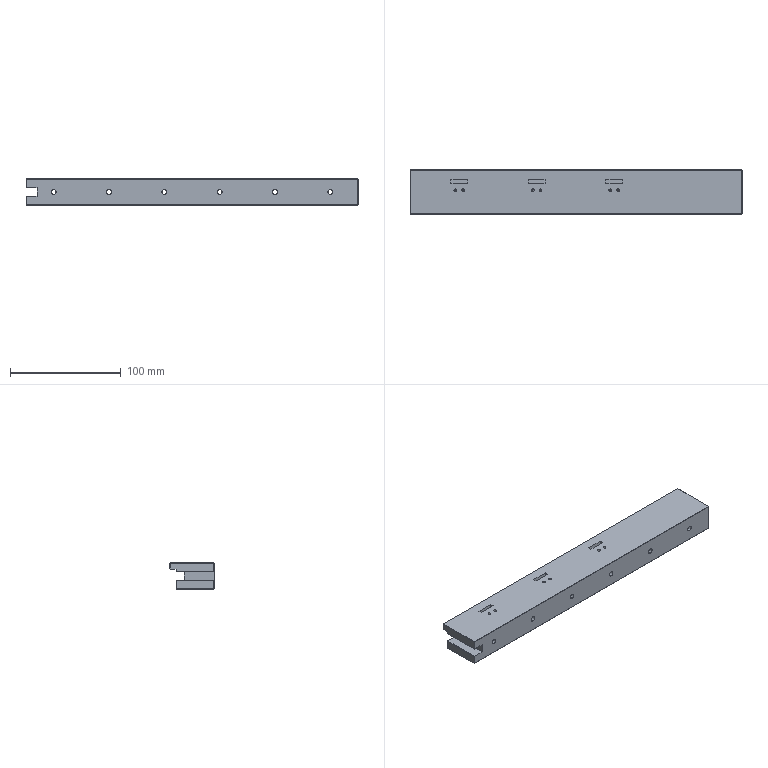Part | STEP file | Semi-finished track | 1 solid | 109 faces | box 300 x 40 x 24 mm | volume 231580 mm3 | plane 61 | cylinder 36 | cone 12 | commonest cylinder face diameters 2.5 x12 4.5 x12 7.5 x12